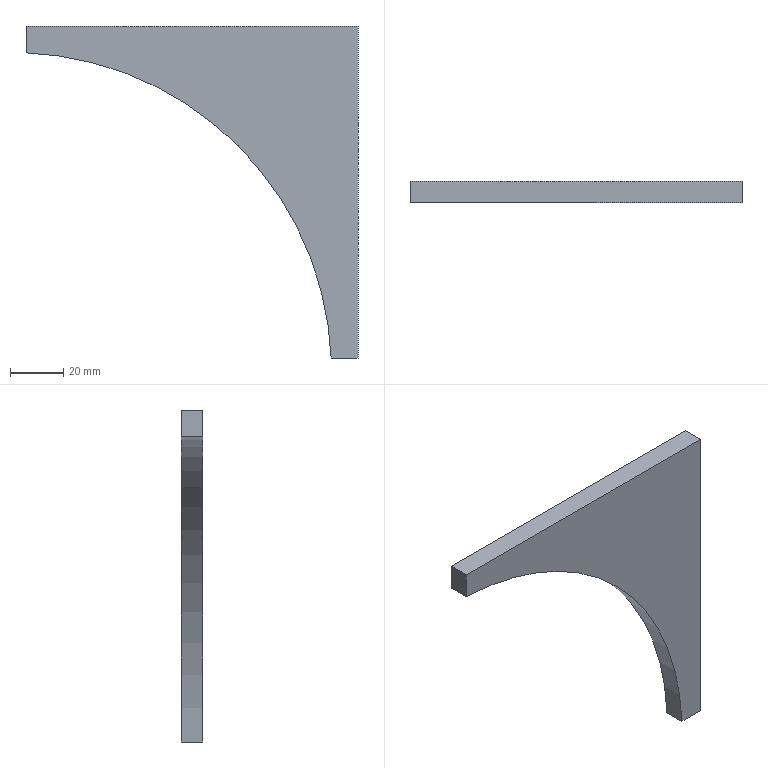Part | SolidWorks | features Extrusion 1 | 1 solid | 7 faces | box 125 x 8 x 125 mm | volume 43919 mm3 | plane 6 | cylinder 1 | commonest cylinder face diameters 240 x1
STEP:
#1=CARTESIAN_POINT('',(-125.,0.,-10.104));
#2=VERTEX_POINT('',#1);
#3=CARTESIAN_POINT('',(-125.,0.,0.));
#4=VERTEX_POINT('',#3);
#5=CARTESIAN_POINT('',(-125.,0.,0.));
#6=DIRECTION('',(0.,0.,1.));
#7=VECTOR('',#6,1000.);
#8=LINE('',#5,#7);
#9=EDGE_CURVE('',#2,#4,#8,.T.);
#10=ORIENTED_EDGE('',*,*,#9,.T.);
#11=CARTESIAN_POINT('',(-125.,8.,0.));
#12=VERTEX_POINT('',#11);
#13=CARTESIAN_POINT('',(-125.,8.,0.));
#14=DIRECTION('',(0.,-1.,0.));
#15=VECTOR('',#14,1000.);
#16=LINE('',#13,#15);
#17=EDGE_CURVE('',#12,#4,#16,.T.);
#18=ORIENTED_EDGE('',*,*,#17,.F.);
#19=CARTESIAN_POINT('',(-125.,8.,-10.104));
#20=VERTEX_POINT('',#19);
#21=CARTESIAN_POINT('',(-125.,8.,0.));
#22=DIRECTION('',(0.,0.,1.));
#23=VECTOR('',#22,1000.);
#24=LINE('',#21,#23);
#25=EDGE_CURVE('',#20,#12,#24,.T.);
#26=ORIENTED_EDGE('',*,*,#25,.F.);
#27=CARTESIAN_POINT('',(-125.,8.,-10.104));
#28=DIRECTION('',(0.,-1.,0.));
#29=VECTOR('',#28,1000.);
#30=LINE('',#27,#29);
#31=EDGE_CURVE('',#20,#2,#30,.T.);
#32=ORIENTED_EDGE('',*,*,#31,.T.);
#33=EDGE_LOOP('',(#10,#18,#26,#32));
#34=FACE_OUTER_BOUND('',#33,.T.);
#35=CARTESIAN_POINT('',(-125.,8.,0.));
#36=DIRECTION('',(1.,0.,0.));
#37=DIRECTION('',(0.,0.,-1.));
#38=AXIS2_PLACEMENT_3D('',#35,#36,#37);
#39=PLANE('',#38);
#40=ADVANCED_FACE('',(#34),#39,.F.);
#41=CARTESIAN_POINT('',(0.,0.,0.));
#42=VERTEX_POINT('',#41);
#43=CARTESIAN_POINT('',(-125.,0.,0.));
#44=DIRECTION('',(1.,0.,0.));
#45=VECTOR('',#44,1000.);
#46=LINE('',#43,#45);
#47=EDGE_CURVE('',#4,#42,#46,.T.);
#48=ORIENTED_EDGE('',*,*,#47,.T.);
#49=CARTESIAN_POINT('',(0.,8.,0.));
#50=VERTEX_POINT('',#49);
#51=CARTESIAN_POINT('',(0.,8.,0.));
#52=DIRECTION('',(0.,-1.,0.));
#53=VECTOR('',#52,1000.);
#54=LINE('',#51,#53);
#55=EDGE_CURVE('',#50,#42,#54,.T.);
#56=ORIENTED_EDGE('',*,*,#55,.F.);
#57=CARTESIAN_POINT('',(-125.,8.,0.));
#58=DIRECTION('',(1.,0.,0.));
#59=VECTOR('',#58,1000.);
#60=LINE('',#57,#59);
#61=EDGE_CURVE('',#12,#50,#60,.T.);
#62=ORIENTED_EDGE('',*,*,#61,.F.);
#63=ORIENTED_EDGE('',*,*,#17,.T.);
#64=EDGE_LOOP('',(#48,#56,#62,#63));
#65=FACE_OUTER_BOUND('',#64,.T.);
#66=CARTESIAN_POINT('',(-125.,8.,0.));
#67=DIRECTION('',(0.,0.,-1.));
#68=DIRECTION('',(-1.,0.,0.));
#69=AXIS2_PLACEMENT_3D('',#66,#67,#68);
#70=PLANE('',#69);
#71=ADVANCED_FACE('',(#65),#70,.F.);
#72=CARTESIAN_POINT('',(0.,0.,-125.));
#73=VERTEX_POINT('',#72);
#74=CARTESIAN_POINT('',(0.,0.,0.));
#75=DIRECTION('',(0.,0.,-1.));
#76=VECTOR('',#75,1000.);
#77=LINE('',#74,#76);
#78=EDGE_CURVE('',#42,#73,#77,.T.);
#79=ORIENTED_EDGE('',*,*,#78,.T.);
#80=CARTESIAN_POINT('',(0.,8.,-125.));
#81=VERTEX_POINT('',#80);
#82=CARTESIAN_POINT('',(0.,8.,-125.));
#83=DIRECTION('',(0.,-1.,0.));
#84=VECTOR('',#83,1000.);
#85=LINE('',#82,#84);
#86=EDGE_CURVE('',#81,#73,#85,.T.);
#87=ORIENTED_EDGE('',*,*,#86,.F.);
#88=CARTESIAN_POINT('',(0.,8.,0.));
#89=DIRECTION('',(0.,0.,-1.));
#90=VECTOR('',#89,1000.);
#91=LINE('',#88,#90);
#92=EDGE_CURVE('',#50,#81,#91,.T.);
#93=ORIENTED_EDGE('',*,*,#92,.F.);
#94=ORIENTED_EDGE('',*,*,#55,.T.);
#95=EDGE_LOOP('',(#79,#87,#93,#94));
#96=FACE_OUTER_BOUND('',#95,.T.);
#97=CARTESIAN_POINT('',(0.,8.,0.));
#98=DIRECTION('',(-1.,0.,0.));
#99=DIRECTION('',(0.,0.,1.));
#100=AXIS2_PLACEMENT_3D('',#97,#98,#99);
#101=PLANE('',#100);
#102=ADVANCED_FACE('',(#96),#101,.F.);
#103=CARTESIAN_POINT('',(-10.104,0.,-125.));
#104=VERTEX_POINT('',#103);
#105=CARTESIAN_POINT('',(0.,0.,-125.));
#106=DIRECTION('',(-1.,0.,0.));
#107=VECTOR('',#106,1000.);
#108=LINE('',#105,#107);
#109=EDGE_CURVE('',#73,#104,#108,.T.);
#110=ORIENTED_EDGE('',*,*,#109,.T.);
#111=CARTESIAN_POINT('',(-10.104,8.,-125.));
#112=VERTEX_POINT('',#111);
#113=CARTESIAN_POINT('',(-10.104,8.,-125.));
#114=DIRECTION('',(0.,-1.,0.));
#115=VECTOR('',#114,1000.);
#116=LINE('',#113,#115);
#117=EDGE_CURVE('',#112,#104,#116,.T.);
#118=ORIENTED_EDGE('',*,*,#117,.F.);
#119=CARTESIAN_POINT('',(0.,8.,-125.));
#120=DIRECTION('',(-1.,0.,0.));
#121=VECTOR('',#120,1000.);
#122=LINE('',#119,#121);
#123=EDGE_CURVE('',#81,#112,#122,.T.);
#124=ORIENTED_EDGE('',*,*,#123,.F.);
#125=ORIENTED_EDGE('',*,*,#86,.T.);
#126=EDGE_LOOP('',(#110,#118,#124,#125));
#127=FACE_OUTER_BOUND('',#126,.T.);
#128=CARTESIAN_POINT('',(0.,8.,-125.));
#129=DIRECTION('',(0.,0.,1.));
#130=DIRECTION('',(1.,0.,0.));
#131=AXIS2_PLACEMENT_3D('',#128,#129,#130);
#132=PLANE('',#131);
#133=ADVANCED_FACE('',(#127),#132,.F.);
#134=CARTESIAN_POINT('',(-130.,0.,-130.));
#135=DIRECTION('',(0.,-1.,0.));
#136=DIRECTION('',(0.,0.,1.));
#137=AXIS2_PLACEMENT_3D('',#134,#135,#136);
#138=CIRCLE('',#137,120.);
#139=EDGE_CURVE('',#104,#2,#138,.T.);
#140=ORIENTED_EDGE('',*,*,#139,.T.);
#141=ORIENTED_EDGE('',*,*,#31,.F.);
#142=CARTESIAN_POINT('',(-130.,8.,-130.));
#143=DIRECTION('',(0.,-1.,0.));
#144=DIRECTION('',(0.,0.,1.));
#145=AXIS2_PLACEMENT_3D('',#142,#143,#144);
#146=CIRCLE('',#145,120.);
#147=EDGE_CURVE('',#112,#20,#146,.T.);
#148=ORIENTED_EDGE('',*,*,#147,.F.);
#149=ORIENTED_EDGE('',*,*,#117,.T.);
#150=EDGE_LOOP('',(#140,#141,#148,#149));
#151=FACE_OUTER_BOUND('',#150,.T.);
#152=CARTESIAN_POINT('',(-130.,8.,-130.));
#153=DIRECTION('',(0.,-1.,0.));
#154=DIRECTION('',(0.,0.,-1.));
#155=AXIS2_PLACEMENT_3D('',#152,#153,#154);
#156=CYLINDRICAL_SURFACE('',#155,120.);
#157=ADVANCED_FACE('',(#151),#156,.F.);
#158=ORIENTED_EDGE('',*,*,#25,.T.);
#159=ORIENTED_EDGE('',*,*,#61,.T.);
#160=ORIENTED_EDGE('',*,*,#92,.T.);
#161=ORIENTED_EDGE('',*,*,#123,.T.);
#162=ORIENTED_EDGE('',*,*,#147,.T.);
#163=EDGE_LOOP('',(#158,#159,#160,#161,#162));
#164=FACE_OUTER_BOUND('',#163,.T.);
#165=CARTESIAN_POINT('',(-130.,8.,-130.));
#166=DIRECTION('',(0.,1.,0.));
#167=DIRECTION('',(0.,0.,1.));
#168=AXIS2_PLACEMENT_3D('',#165,#166,#167);
#169=PLANE('',#168);
#170=ADVANCED_FACE('',(#164),#169,.T.);
#171=ORIENTED_EDGE('',*,*,#9,.F.);
#172=ORIENTED_EDGE('',*,*,#139,.F.);
#173=ORIENTED_EDGE('',*,*,#109,.F.);
#174=ORIENTED_EDGE('',*,*,#78,.F.);
#175=ORIENTED_EDGE('',*,*,#47,.F.);
#176=EDGE_LOOP('',(#171,#172,#173,#174,#175));
#177=FACE_OUTER_BOUND('',#176,.T.);
#178=CARTESIAN_POINT('',(-130.,0.,-130.));
#179=DIRECTION('',(0.,1.,0.));
#180=DIRECTION('',(0.,0.,1.));
#181=AXIS2_PLACEMENT_3D('',#178,#179,#180);
#182=PLANE('',#181);
#183=ADVANCED_FACE('',(#177),#182,.F.);
#184=CLOSED_SHELL('',(#40,#71,#102,#133,#157,#170,#183));
#185=MANIFOLD_SOLID_BREP('',#184);
#186=CARTESIAN_POINT('',(0.,0.,0.));
#187=DIRECTION('',(0.,0.,1.));
#188=DIRECTION('',(1.,0.,0.));
#189=AXIS2_PLACEMENT_3D('',#186,#187,#188);
#190=(LENGTH_UNIT()NAMED_UNIT(*)SI_UNIT(.MILLI.,.METRE.));
#191=UNCERTAINTY_MEASURE_WITH_UNIT(LENGTH_MEASURE(0.00001),#190,'','');
#192=(NAMED_UNIT(*)PLANE_ANGLE_UNIT()SI_UNIT($,.RADIAN.));
#193=(NAMED_UNIT(*)SI_UNIT($,.STERADIAN.)SOLID_ANGLE_UNIT());
#194=(GEOMETRIC_REPRESENTATION_CONTEXT(3)GLOBAL_UNCERTAINTY_ASSIGNED_CONTEXT((#191))GLOBAL_UNIT_ASSIGNED_CONTEXT((#190,#192,#193))REPRESENTATION_CONTEXT('',''));
#195=ADVANCED_BREP_SHAPE_REPRESENTATION('',(#185,#189),#194);